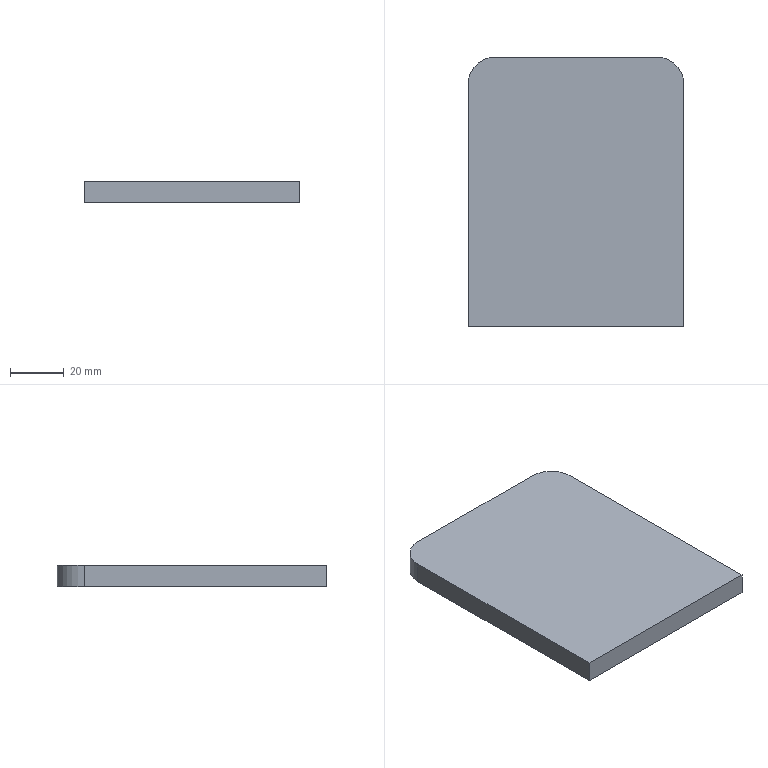Part | SolidWorks | features Extrusion 1, Fillet 1 | 1 solid | 8 faces | box 80 x 100 x 8 mm | volume 63657 mm3 | plane 6 | cylinder 2 | commonest cylinder face diameters 20 x2
STEP:
#1=CARTESIAN_POINT('',(0.,-10.,8.));
#2=VERTEX_POINT('',#1);
#3=CARTESIAN_POINT('',(0.,-100.,8.));
#4=VERTEX_POINT('',#3);
#5=CARTESIAN_POINT('',(0.,0.,8.));
#6=DIRECTION('',(0.,-1.,0.));
#7=VECTOR('',#6,1000.);
#8=LINE('',#5,#7);
#9=EDGE_CURVE('',#2,#4,#8,.T.);
#10=ORIENTED_EDGE('',*,*,#9,.F.);
#11=CARTESIAN_POINT('',(0.,-10.,0.));
#12=VERTEX_POINT('',#11);
#13=CARTESIAN_POINT('',(0.,-10.,8.));
#14=DIRECTION('',(0.,0.,-1.));
#15=VECTOR('',#14,1000.);
#16=LINE('',#13,#15);
#17=EDGE_CURVE('',#2,#12,#16,.T.);
#18=ORIENTED_EDGE('',*,*,#17,.T.);
#19=CARTESIAN_POINT('',(0.,-100.,0.));
#20=VERTEX_POINT('',#19);
#21=CARTESIAN_POINT('',(0.,0.,0.));
#22=DIRECTION('',(0.,-1.,0.));
#23=VECTOR('',#22,1000.);
#24=LINE('',#21,#23);
#25=EDGE_CURVE('',#12,#20,#24,.T.);
#26=ORIENTED_EDGE('',*,*,#25,.T.);
#27=CARTESIAN_POINT('',(0.,-100.,8.));
#28=DIRECTION('',(0.,0.,-1.));
#29=VECTOR('',#28,1000.);
#30=LINE('',#27,#29);
#31=EDGE_CURVE('',#4,#20,#30,.T.);
#32=ORIENTED_EDGE('',*,*,#31,.F.);
#33=EDGE_LOOP('',(#10,#18,#26,#32));
#34=FACE_OUTER_BOUND('',#33,.T.);
#35=CARTESIAN_POINT('',(0.,0.,8.));
#36=DIRECTION('',(1.,0.,0.));
#37=DIRECTION('',(0.,1.,0.));
#38=AXIS2_PLACEMENT_3D('',#35,#36,#37);
#39=PLANE('',#38);
#40=ADVANCED_FACE('',(#34),#39,.F.);
#41=CARTESIAN_POINT('',(80.,-100.,0.));
#42=VERTEX_POINT('',#41);
#43=CARTESIAN_POINT('',(0.,-100.,0.));
#44=DIRECTION('',(1.,0.,0.));
#45=VECTOR('',#44,1000.);
#46=LINE('',#43,#45);
#47=EDGE_CURVE('',#20,#42,#46,.T.);
#48=ORIENTED_EDGE('',*,*,#47,.T.);
#49=CARTESIAN_POINT('',(80.,-100.,8.));
#50=VERTEX_POINT('',#49);
#51=CARTESIAN_POINT('',(80.,-100.,8.));
#52=DIRECTION('',(0.,0.,-1.));
#53=VECTOR('',#52,1000.);
#54=LINE('',#51,#53);
#55=EDGE_CURVE('',#50,#42,#54,.T.);
#56=ORIENTED_EDGE('',*,*,#55,.F.);
#57=CARTESIAN_POINT('',(0.,-100.,8.));
#58=DIRECTION('',(1.,0.,0.));
#59=VECTOR('',#58,1000.);
#60=LINE('',#57,#59);
#61=EDGE_CURVE('',#4,#50,#60,.T.);
#62=ORIENTED_EDGE('',*,*,#61,.F.);
#63=ORIENTED_EDGE('',*,*,#31,.T.);
#64=EDGE_LOOP('',(#48,#56,#62,#63));
#65=FACE_OUTER_BOUND('',#64,.T.);
#66=CARTESIAN_POINT('',(0.,-100.,8.));
#67=DIRECTION('',(0.,1.,0.));
#68=DIRECTION('',(0.,0.,1.));
#69=AXIS2_PLACEMENT_3D('',#66,#67,#68);
#70=PLANE('',#69);
#71=ADVANCED_FACE('',(#65),#70,.F.);
#72=CARTESIAN_POINT('',(80.,-10.,0.));
#73=VERTEX_POINT('',#72);
#74=CARTESIAN_POINT('',(80.,0.,0.));
#75=DIRECTION('',(0.,1.,0.));
#76=VECTOR('',#75,1000.);
#77=LINE('',#74,#76);
#78=EDGE_CURVE('',#42,#73,#77,.T.);
#79=ORIENTED_EDGE('',*,*,#78,.T.);
#80=CARTESIAN_POINT('',(80.,-10.,8.));
#81=VERTEX_POINT('',#80);
#82=CARTESIAN_POINT('',(80.,-10.,8.));
#83=DIRECTION('',(0.,0.,1.));
#84=VECTOR('',#83,1000.);
#85=LINE('',#82,#84);
#86=EDGE_CURVE('',#73,#81,#85,.T.);
#87=ORIENTED_EDGE('',*,*,#86,.T.);
#88=CARTESIAN_POINT('',(80.,0.,8.));
#89=DIRECTION('',(0.,1.,0.));
#90=VECTOR('',#89,1000.);
#91=LINE('',#88,#90);
#92=EDGE_CURVE('',#50,#81,#91,.T.);
#93=ORIENTED_EDGE('',*,*,#92,.F.);
#94=ORIENTED_EDGE('',*,*,#55,.T.);
#95=EDGE_LOOP('',(#79,#87,#93,#94));
#96=FACE_OUTER_BOUND('',#95,.T.);
#97=CARTESIAN_POINT('',(80.,0.,8.));
#98=DIRECTION('',(-1.,0.,0.));
#99=DIRECTION('',(0.,-1.,0.));
#100=AXIS2_PLACEMENT_3D('',#97,#98,#99);
#101=PLANE('',#100);
#102=ADVANCED_FACE('',(#96),#101,.F.);
#103=CARTESIAN_POINT('',(70.,0.,0.));
#104=VERTEX_POINT('',#103);
#105=CARTESIAN_POINT('',(10.,0.,0.));
#106=VERTEX_POINT('',#105);
#107=CARTESIAN_POINT('',(0.,0.,0.));
#108=DIRECTION('',(-1.,0.,0.));
#109=VECTOR('',#108,1000.);
#110=LINE('',#107,#109);
#111=EDGE_CURVE('',#104,#106,#110,.T.);
#112=ORIENTED_EDGE('',*,*,#111,.T.);
#113=CARTESIAN_POINT('',(10.,0.,8.));
#114=VERTEX_POINT('',#113);
#115=CARTESIAN_POINT('',(10.,0.,8.));
#116=DIRECTION('',(0.,0.,1.));
#117=VECTOR('',#116,1000.);
#118=LINE('',#115,#117);
#119=EDGE_CURVE('',#106,#114,#118,.T.);
#120=ORIENTED_EDGE('',*,*,#119,.T.);
#121=CARTESIAN_POINT('',(70.,0.,8.));
#122=VERTEX_POINT('',#121);
#123=CARTESIAN_POINT('',(0.,0.,8.));
#124=DIRECTION('',(-1.,0.,0.));
#125=VECTOR('',#124,1000.);
#126=LINE('',#123,#125);
#127=EDGE_CURVE('',#122,#114,#126,.T.);
#128=ORIENTED_EDGE('',*,*,#127,.F.);
#129=CARTESIAN_POINT('',(70.,0.,8.));
#130=DIRECTION('',(0.,0.,-1.));
#131=VECTOR('',#130,1000.);
#132=LINE('',#129,#131);
#133=EDGE_CURVE('',#122,#104,#132,.T.);
#134=ORIENTED_EDGE('',*,*,#133,.T.);
#135=EDGE_LOOP('',(#112,#120,#128,#134));
#136=FACE_OUTER_BOUND('',#135,.T.);
#137=CARTESIAN_POINT('',(0.,0.,8.));
#138=DIRECTION('',(0.,-1.,0.));
#139=DIRECTION('',(0.,0.,-1.));
#140=AXIS2_PLACEMENT_3D('',#137,#138,#139);
#141=PLANE('',#140);
#142=ADVANCED_FACE('',(#136),#141,.F.);
#143=ORIENTED_EDGE('',*,*,#127,.T.);
#144=CARTESIAN_POINT('',(10.,-10.,8.));
#145=DIRECTION('',(0.,0.,1.));
#146=DIRECTION('',(1.,0.,0.));
#147=AXIS2_PLACEMENT_3D('',#144,#145,#146);
#148=CIRCLE('',#147,10.);
#149=EDGE_CURVE('',#114,#2,#148,.T.);
#150=ORIENTED_EDGE('',*,*,#149,.T.);
#151=ORIENTED_EDGE('',*,*,#9,.T.);
#152=ORIENTED_EDGE('',*,*,#61,.T.);
#153=ORIENTED_EDGE('',*,*,#92,.T.);
#154=CARTESIAN_POINT('',(70.,-10.,8.));
#155=DIRECTION('',(0.,0.,1.));
#156=DIRECTION('',(1.,0.,0.));
#157=AXIS2_PLACEMENT_3D('',#154,#155,#156);
#158=CIRCLE('',#157,10.);
#159=EDGE_CURVE('',#81,#122,#158,.T.);
#160=ORIENTED_EDGE('',*,*,#159,.T.);
#161=EDGE_LOOP('',(#143,#150,#151,#152,#153,#160));
#162=FACE_OUTER_BOUND('',#161,.T.);
#163=CARTESIAN_POINT('',(0.,0.,8.));
#164=DIRECTION('',(0.,0.,1.));
#165=DIRECTION('',(1.,0.,0.));
#166=AXIS2_PLACEMENT_3D('',#163,#164,#165);
#167=PLANE('',#166);
#168=ADVANCED_FACE('',(#162),#167,.T.);
#169=ORIENTED_EDGE('',*,*,#25,.F.);
#170=CARTESIAN_POINT('',(10.,-10.,0.));
#171=DIRECTION('',(0.,0.,-1.));
#172=DIRECTION('',(1.,0.,0.));
#173=AXIS2_PLACEMENT_3D('',#170,#171,#172);
#174=CIRCLE('',#173,10.);
#175=EDGE_CURVE('',#12,#106,#174,.T.);
#176=ORIENTED_EDGE('',*,*,#175,.T.);
#177=ORIENTED_EDGE('',*,*,#111,.F.);
#178=CARTESIAN_POINT('',(70.,-10.,0.));
#179=DIRECTION('',(0.,0.,-1.));
#180=DIRECTION('',(1.,0.,0.));
#181=AXIS2_PLACEMENT_3D('',#178,#179,#180);
#182=CIRCLE('',#181,10.);
#183=EDGE_CURVE('',#104,#73,#182,.T.);
#184=ORIENTED_EDGE('',*,*,#183,.T.);
#185=ORIENTED_EDGE('',*,*,#78,.F.);
#186=ORIENTED_EDGE('',*,*,#47,.F.);
#187=EDGE_LOOP('',(#169,#176,#177,#184,#185,#186));
#188=FACE_OUTER_BOUND('',#187,.T.);
#189=CARTESIAN_POINT('',(0.,0.,0.));
#190=DIRECTION('',(0.,0.,1.));
#191=DIRECTION('',(1.,0.,0.));
#192=AXIS2_PLACEMENT_3D('',#189,#190,#191);
#193=PLANE('',#192);
#194=ADVANCED_FACE('',(#188),#193,.F.);
#195=ORIENTED_EDGE('',*,*,#149,.F.);
#196=ORIENTED_EDGE('',*,*,#119,.F.);
#197=ORIENTED_EDGE('',*,*,#175,.F.);
#198=ORIENTED_EDGE('',*,*,#17,.F.);
#199=EDGE_LOOP('',(#195,#196,#197,#198));
#200=FACE_OUTER_BOUND('',#199,.T.);
#201=CARTESIAN_POINT('',(10.,-10.,8.));
#202=DIRECTION('',(0.,0.,-1.));
#203=DIRECTION('',(-1.,0.,0.));
#204=AXIS2_PLACEMENT_3D('',#201,#202,#203);
#205=CYLINDRICAL_SURFACE('',#204,10.);
#206=ADVANCED_FACE('',(#200),#205,.T.);
#207=ORIENTED_EDGE('',*,*,#159,.F.);
#208=ORIENTED_EDGE('',*,*,#86,.F.);
#209=ORIENTED_EDGE('',*,*,#183,.F.);
#210=ORIENTED_EDGE('',*,*,#133,.F.);
#211=EDGE_LOOP('',(#207,#208,#209,#210));
#212=FACE_OUTER_BOUND('',#211,.T.);
#213=CARTESIAN_POINT('',(70.,-10.,8.));
#214=DIRECTION('',(0.,0.,-1.));
#215=DIRECTION('',(-1.,0.,0.));
#216=AXIS2_PLACEMENT_3D('',#213,#214,#215);
#217=CYLINDRICAL_SURFACE('',#216,10.);
#218=ADVANCED_FACE('',(#212),#217,.T.);
#219=CLOSED_SHELL('',(#40,#71,#102,#142,#168,#194,#206,#218));
#220=MANIFOLD_SOLID_BREP('',#219);
#221=CARTESIAN_POINT('',(0.,0.,0.));
#222=DIRECTION('',(0.,0.,1.));
#223=DIRECTION('',(1.,0.,0.));
#224=AXIS2_PLACEMENT_3D('',#221,#222,#223);
#225=(LENGTH_UNIT()NAMED_UNIT(*)SI_UNIT(.MILLI.,.METRE.));
#226=UNCERTAINTY_MEASURE_WITH_UNIT(LENGTH_MEASURE(0.00001),#225,'','');
#227=(NAMED_UNIT(*)PLANE_ANGLE_UNIT()SI_UNIT($,.RADIAN.));
#228=(NAMED_UNIT(*)SI_UNIT($,.STERADIAN.)SOLID_ANGLE_UNIT());
#229=(GEOMETRIC_REPRESENTATION_CONTEXT(3)GLOBAL_UNCERTAINTY_ASSIGNED_CONTEXT((#226))GLOBAL_UNIT_ASSIGNED_CONTEXT((#225,#227,#228))REPRESENTATION_CONTEXT('',''));
#230=ADVANCED_BREP_SHAPE_REPRESENTATION('',(#220,#224),#229);